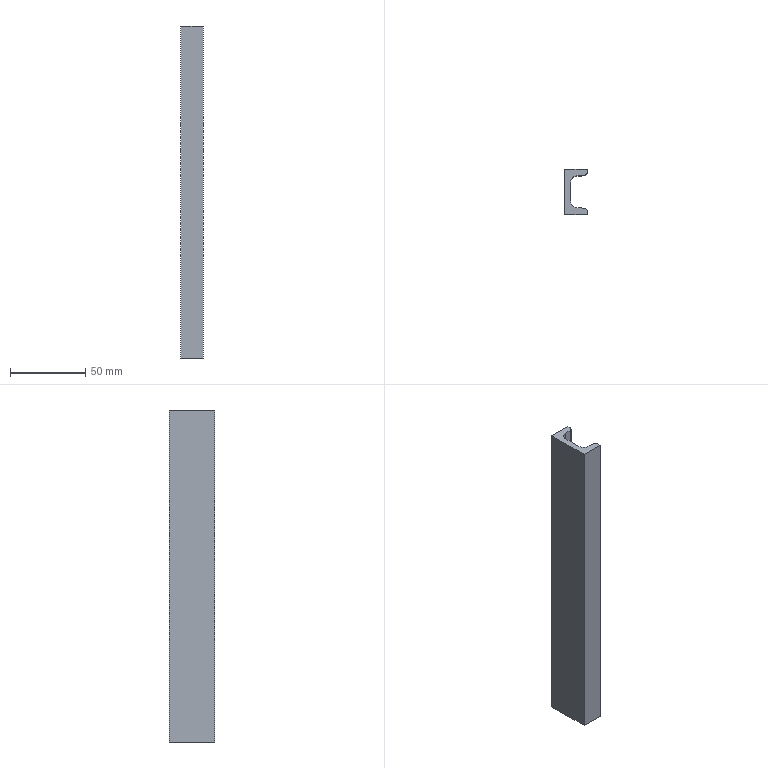Part | STEP file | DIN 1026-1 U 30x15 1785508252631 | 1 solid | 14 faces | box 15 x 30 x 220 mm | volume 48676 mm3 | plane 10 | cylinder 4 | commonest cylinder face diameters 4 x2 9 x2
STEP:
#1=CARTESIAN_POINT('',(4.,-6.066,220.));
#2=VERTEX_POINT('',#1);
#3=CARTESIAN_POINT('',(8.141,-10.551,220.));
#4=VERTEX_POINT('',#3);
#5=CARTESIAN_POINT('',(8.5,-6.066,220.));
#6=DIRECTION('',(0.,0.,1.));
#7=DIRECTION('',(-1.,0.,0.));
#8=AXIS2_PLACEMENT_3D('',#5,#6,#7);
#9=CIRCLE('',#8,4.5);
#10=EDGE_CURVE('',#2,#4,#9,.T.);
#11=ORIENTED_EDGE('',*,*,#10,.T.);
#12=CARTESIAN_POINT('',(8.141,-10.551,0.));
#13=VERTEX_POINT('',#12);
#14=CARTESIAN_POINT('',(8.141,-10.551,0.));
#15=DIRECTION('',(0.,0.,1.));
#16=VECTOR('',#15,10.);
#17=LINE('',#14,#16);
#18=EDGE_CURVE('',#13,#4,#17,.T.);
#19=ORIENTED_EDGE('',*,*,#18,.F.);
#20=CARTESIAN_POINT('',(4.,-6.066,0.));
#21=VERTEX_POINT('',#20);
#22=CARTESIAN_POINT('',(8.5,-6.066,0.));
#23=DIRECTION('',(0.,0.,1.));
#24=DIRECTION('',(-1.,0.,0.));
#25=AXIS2_PLACEMENT_3D('',#22,#23,#24);
#26=CIRCLE('',#25,4.5);
#27=EDGE_CURVE('',#21,#13,#26,.T.);
#28=ORIENTED_EDGE('',*,*,#27,.F.);
#29=CARTESIAN_POINT('',(4.,-6.066,0.));
#30=DIRECTION('',(0.,0.,1.));
#31=VECTOR('',#30,10.);
#32=LINE('',#29,#31);
#33=EDGE_CURVE('',#21,#2,#32,.T.);
#34=ORIENTED_EDGE('',*,*,#33,.T.);
#35=EDGE_LOOP('',(#11,#19,#28,#34));
#36=FACE_OUTER_BOUND('',#35,.T.);
#37=CARTESIAN_POINT('',(8.5,-6.066,0.));
#38=DIRECTION('',(0.,0.,1.));
#39=DIRECTION('',(-1.,0.,0.));
#40=AXIS2_PLACEMENT_3D('',#37,#38,#39);
#41=CYLINDRICAL_SURFACE('',#40,4.5);
#42=ADVANCED_FACE('',(#36),#41,.F.);
#43=CARTESIAN_POINT('',(13.159,-10.953,220.));
#44=VERTEX_POINT('',#43);
#45=CARTESIAN_POINT('',(7.403,-10.492,220.));
#46=DIRECTION('',(0.9968,-0.07975,0.));
#47=VECTOR('',#46,10.);
#48=LINE('',#45,#47);
#49=EDGE_CURVE('',#4,#44,#48,.T.);
#50=ORIENTED_EDGE('',*,*,#49,.T.);
#51=CARTESIAN_POINT('',(13.159,-10.953,0.));
#52=VERTEX_POINT('',#51);
#53=CARTESIAN_POINT('',(13.159,-10.953,0.));
#54=DIRECTION('',(0.,0.,1.));
#55=VECTOR('',#54,10.);
#56=LINE('',#53,#55);
#57=EDGE_CURVE('',#52,#44,#56,.T.);
#58=ORIENTED_EDGE('',*,*,#57,.F.);
#59=CARTESIAN_POINT('',(7.403,-10.492,0.));
#60=DIRECTION('',(0.9968,-0.07975,0.));
#61=VECTOR('',#60,10.);
#62=LINE('',#59,#61);
#63=EDGE_CURVE('',#13,#52,#62,.T.);
#64=ORIENTED_EDGE('',*,*,#63,.F.);
#65=ORIENTED_EDGE('',*,*,#18,.T.);
#66=EDGE_LOOP('',(#50,#58,#64,#65));
#67=FACE_OUTER_BOUND('',#66,.T.);
#68=CARTESIAN_POINT('',(8.141,-10.551,0.));
#69=DIRECTION('',(0.07975,0.9968,0.));
#70=DIRECTION('',(0.,0.,1.));
#71=AXIS2_PLACEMENT_3D('',#68,#69,#70);
#72=PLANE('',#71);
#73=ADVANCED_FACE('',(#67),#72,.T.);
#74=CARTESIAN_POINT('',(15.,-12.946,220.));
#75=VERTEX_POINT('',#74);
#76=CARTESIAN_POINT('',(13.,-12.946,220.));
#77=DIRECTION('',(0.,0.,-1.));
#78=DIRECTION('',(-1.,0.,0.));
#79=AXIS2_PLACEMENT_3D('',#76,#77,#78);
#80=CIRCLE('',#79,2.);
#81=EDGE_CURVE('',#44,#75,#80,.T.);
#82=ORIENTED_EDGE('',*,*,#81,.T.);
#83=CARTESIAN_POINT('',(15.,-12.946,0.));
#84=VERTEX_POINT('',#83);
#85=CARTESIAN_POINT('',(15.,-12.946,0.));
#86=DIRECTION('',(0.,0.,1.));
#87=VECTOR('',#86,10.);
#88=LINE('',#85,#87);
#89=EDGE_CURVE('',#84,#75,#88,.T.);
#90=ORIENTED_EDGE('',*,*,#89,.F.);
#91=CARTESIAN_POINT('',(13.,-12.946,0.));
#92=DIRECTION('',(0.,0.,-1.));
#93=DIRECTION('',(-1.,0.,0.));
#94=AXIS2_PLACEMENT_3D('',#91,#92,#93);
#95=CIRCLE('',#94,2.);
#96=EDGE_CURVE('',#52,#84,#95,.T.);
#97=ORIENTED_EDGE('',*,*,#96,.F.);
#98=ORIENTED_EDGE('',*,*,#57,.T.);
#99=EDGE_LOOP('',(#82,#90,#97,#98));
#100=FACE_OUTER_BOUND('',#99,.T.);
#101=CARTESIAN_POINT('',(13.,-12.946,0.));
#102=DIRECTION('',(0.,0.,1.));
#103=DIRECTION('',(-1.,0.,0.));
#104=AXIS2_PLACEMENT_3D('',#101,#102,#103);
#105=CYLINDRICAL_SURFACE('',#104,2.);
#106=ADVANCED_FACE('',(#100),#105,.T.);
#107=CARTESIAN_POINT('',(15.,-15.,220.));
#108=VERTEX_POINT('',#107);
#109=CARTESIAN_POINT('',(15.,-6.473,220.));
#110=DIRECTION('',(0.,-1.,0.));
#111=VECTOR('',#110,10.);
#112=LINE('',#109,#111);
#113=EDGE_CURVE('',#75,#108,#112,.T.);
#114=ORIENTED_EDGE('',*,*,#113,.T.);
#115=CARTESIAN_POINT('',(15.,-15.,0.));
#116=VERTEX_POINT('',#115);
#117=CARTESIAN_POINT('',(15.,-15.,0.));
#118=DIRECTION('',(0.,0.,1.));
#119=VECTOR('',#118,10.);
#120=LINE('',#117,#119);
#121=EDGE_CURVE('',#116,#108,#120,.T.);
#122=ORIENTED_EDGE('',*,*,#121,.F.);
#123=CARTESIAN_POINT('',(15.,-6.473,0.));
#124=DIRECTION('',(0.,-1.,0.));
#125=VECTOR('',#124,10.);
#126=LINE('',#123,#125);
#127=EDGE_CURVE('',#84,#116,#126,.T.);
#128=ORIENTED_EDGE('',*,*,#127,.F.);
#129=ORIENTED_EDGE('',*,*,#89,.T.);
#130=EDGE_LOOP('',(#114,#122,#128,#129));
#131=FACE_OUTER_BOUND('',#130,.T.);
#132=CARTESIAN_POINT('',(15.,-12.946,0.));
#133=DIRECTION('',(1.,0.,0.));
#134=DIRECTION('',(0.,0.,-1.));
#135=AXIS2_PLACEMENT_3D('',#132,#133,#134);
#136=PLANE('',#135);
#137=ADVANCED_FACE('',(#131),#136,.T.);
#138=CARTESIAN_POINT('',(0.,-15.,220.));
#139=VERTEX_POINT('',#138);
#140=CARTESIAN_POINT('',(11.25,-15.,220.));
#141=DIRECTION('',(-1.,0.,0.));
#142=VECTOR('',#141,10.);
#143=LINE('',#140,#142);
#144=EDGE_CURVE('',#108,#139,#143,.T.);
#145=ORIENTED_EDGE('',*,*,#144,.T.);
#146=CARTESIAN_POINT('',(0.,-15.,0.));
#147=VERTEX_POINT('',#146);
#148=CARTESIAN_POINT('',(0.,-15.,0.));
#149=DIRECTION('',(0.,0.,1.));
#150=VECTOR('',#149,10.);
#151=LINE('',#148,#150);
#152=EDGE_CURVE('',#147,#139,#151,.T.);
#153=ORIENTED_EDGE('',*,*,#152,.F.);
#154=CARTESIAN_POINT('',(11.25,-15.,0.));
#155=DIRECTION('',(-1.,0.,0.));
#156=VECTOR('',#155,10.);
#157=LINE('',#154,#156);
#158=EDGE_CURVE('',#116,#147,#157,.T.);
#159=ORIENTED_EDGE('',*,*,#158,.F.);
#160=ORIENTED_EDGE('',*,*,#121,.T.);
#161=EDGE_LOOP('',(#145,#153,#159,#160));
#162=FACE_OUTER_BOUND('',#161,.T.);
#163=CARTESIAN_POINT('',(15.,-15.,0.));
#164=DIRECTION('',(0.,-1.,0.));
#165=DIRECTION('',(0.,0.,-1.));
#166=AXIS2_PLACEMENT_3D('',#163,#164,#165);
#167=PLANE('',#166);
#168=ADVANCED_FACE('',(#162),#167,.T.);
#169=CARTESIAN_POINT('',(0.,15.,220.));
#170=VERTEX_POINT('',#169);
#171=CARTESIAN_POINT('',(0.,0.,220.));
#172=DIRECTION('',(0.,1.,0.));
#173=VECTOR('',#172,10.);
#174=LINE('',#171,#173);
#175=EDGE_CURVE('',#139,#170,#174,.T.);
#176=ORIENTED_EDGE('',*,*,#175,.T.);
#177=CARTESIAN_POINT('',(0.,15.,0.));
#178=VERTEX_POINT('',#177);
#179=CARTESIAN_POINT('',(0.,15.,0.));
#180=DIRECTION('',(0.,0.,1.));
#181=VECTOR('',#180,10.);
#182=LINE('',#179,#181);
#183=EDGE_CURVE('',#178,#170,#182,.T.);
#184=ORIENTED_EDGE('',*,*,#183,.F.);
#185=CARTESIAN_POINT('',(0.,0.,0.));
#186=DIRECTION('',(0.,1.,0.));
#187=VECTOR('',#186,10.);
#188=LINE('',#185,#187);
#189=EDGE_CURVE('',#147,#178,#188,.T.);
#190=ORIENTED_EDGE('',*,*,#189,.F.);
#191=ORIENTED_EDGE('',*,*,#152,.T.);
#192=EDGE_LOOP('',(#176,#184,#190,#191));
#193=FACE_OUTER_BOUND('',#192,.T.);
#194=CARTESIAN_POINT('',(0.,0.,0.));
#195=DIRECTION('',(-1.,0.,0.));
#196=DIRECTION('',(0.,0.,1.));
#197=AXIS2_PLACEMENT_3D('',#194,#195,#196);
#198=PLANE('',#197);
#199=ADVANCED_FACE('',(#193),#198,.T.);
#200=CARTESIAN_POINT('',(15.,15.,220.));
#201=VERTEX_POINT('',#200);
#202=CARTESIAN_POINT('',(3.75,15.,220.));
#203=DIRECTION('',(1.,0.,0.));
#204=VECTOR('',#203,10.);
#205=LINE('',#202,#204);
#206=EDGE_CURVE('',#170,#201,#205,.T.);
#207=ORIENTED_EDGE('',*,*,#206,.T.);
#208=CARTESIAN_POINT('',(15.,15.,0.));
#209=VERTEX_POINT('',#208);
#210=CARTESIAN_POINT('',(15.,15.,0.));
#211=DIRECTION('',(0.,0.,1.));
#212=VECTOR('',#211,10.);
#213=LINE('',#210,#212);
#214=EDGE_CURVE('',#209,#201,#213,.T.);
#215=ORIENTED_EDGE('',*,*,#214,.F.);
#216=CARTESIAN_POINT('',(3.75,15.,0.));
#217=DIRECTION('',(1.,0.,0.));
#218=VECTOR('',#217,10.);
#219=LINE('',#216,#218);
#220=EDGE_CURVE('',#178,#209,#219,.T.);
#221=ORIENTED_EDGE('',*,*,#220,.F.);
#222=ORIENTED_EDGE('',*,*,#183,.T.);
#223=EDGE_LOOP('',(#207,#215,#221,#222));
#224=FACE_OUTER_BOUND('',#223,.T.);
#225=CARTESIAN_POINT('',(0.,15.,0.));
#226=DIRECTION('',(0.,1.,0.));
#227=DIRECTION('',(0.,0.,1.));
#228=AXIS2_PLACEMENT_3D('',#225,#226,#227);
#229=PLANE('',#228);
#230=ADVANCED_FACE('',(#224),#229,.T.);
#231=CARTESIAN_POINT('',(15.,12.946,220.));
#232=VERTEX_POINT('',#231);
#233=CARTESIAN_POINT('',(15.,7.5,220.));
#234=DIRECTION('',(0.,-1.,0.));
#235=VECTOR('',#234,10.);
#236=LINE('',#233,#235);
#237=EDGE_CURVE('',#201,#232,#236,.T.);
#238=ORIENTED_EDGE('',*,*,#237,.T.);
#239=CARTESIAN_POINT('',(15.,12.946,0.));
#240=VERTEX_POINT('',#239);
#241=CARTESIAN_POINT('',(15.,12.946,0.));
#242=DIRECTION('',(0.,0.,1.));
#243=VECTOR('',#242,10.);
#244=LINE('',#241,#243);
#245=EDGE_CURVE('',#240,#232,#244,.T.);
#246=ORIENTED_EDGE('',*,*,#245,.F.);
#247=CARTESIAN_POINT('',(15.,7.5,0.));
#248=DIRECTION('',(0.,-1.,0.));
#249=VECTOR('',#248,10.);
#250=LINE('',#247,#249);
#251=EDGE_CURVE('',#209,#240,#250,.T.);
#252=ORIENTED_EDGE('',*,*,#251,.F.);
#253=ORIENTED_EDGE('',*,*,#214,.T.);
#254=EDGE_LOOP('',(#238,#246,#252,#253));
#255=FACE_OUTER_BOUND('',#254,.T.);
#256=CARTESIAN_POINT('',(15.,15.,0.));
#257=DIRECTION('',(1.,0.,0.));
#258=DIRECTION('',(0.,0.,-1.));
#259=AXIS2_PLACEMENT_3D('',#256,#257,#258);
#260=PLANE('',#259);
#261=ADVANCED_FACE('',(#255),#260,.T.);
#262=CARTESIAN_POINT('',(13.159,10.953,220.));
#263=VERTEX_POINT('',#262);
#264=CARTESIAN_POINT('',(13.,12.946,220.));
#265=DIRECTION('',(0.,0.,-1.));
#266=DIRECTION('',(-0.07975,0.9968,0.));
#267=AXIS2_PLACEMENT_3D('',#264,#265,#266);
#268=CIRCLE('',#267,2.);
#269=EDGE_CURVE('',#232,#263,#268,.T.);
#270=ORIENTED_EDGE('',*,*,#269,.T.);
#271=CARTESIAN_POINT('',(13.159,10.953,0.));
#272=VERTEX_POINT('',#271);
#273=CARTESIAN_POINT('',(13.159,10.953,0.));
#274=DIRECTION('',(0.,0.,1.));
#275=VECTOR('',#274,10.);
#276=LINE('',#273,#275);
#277=EDGE_CURVE('',#272,#263,#276,.T.);
#278=ORIENTED_EDGE('',*,*,#277,.F.);
#279=CARTESIAN_POINT('',(13.,12.946,0.));
#280=DIRECTION('',(0.,0.,-1.));
#281=DIRECTION('',(-0.07975,0.9968,0.));
#282=AXIS2_PLACEMENT_3D('',#279,#280,#281);
#283=CIRCLE('',#282,2.);
#284=EDGE_CURVE('',#240,#272,#283,.T.);
#285=ORIENTED_EDGE('',*,*,#284,.F.);
#286=ORIENTED_EDGE('',*,*,#245,.T.);
#287=EDGE_LOOP('',(#270,#278,#285,#286));
#288=FACE_OUTER_BOUND('',#287,.T.);
#289=CARTESIAN_POINT('',(13.,12.946,0.));
#290=DIRECTION('',(0.,0.,1.));
#291=DIRECTION('',(-0.07975,0.9968,0.));
#292=AXIS2_PLACEMENT_3D('',#289,#290,#291);
#293=CYLINDRICAL_SURFACE('',#292,2.);
#294=ADVANCED_FACE('',(#288),#293,.T.);
#295=CARTESIAN_POINT('',(8.141,10.551,220.));
#296=VERTEX_POINT('',#295);
#297=CARTESIAN_POINT('',(9.912,10.693,220.));
#298=DIRECTION('',(-0.9968,-0.07975,0.));
#299=VECTOR('',#298,10.);
#300=LINE('',#297,#299);
#301=EDGE_CURVE('',#263,#296,#300,.T.);
#302=ORIENTED_EDGE('',*,*,#301,.T.);
#303=CARTESIAN_POINT('',(8.141,10.551,0.));
#304=VERTEX_POINT('',#303);
#305=CARTESIAN_POINT('',(8.141,10.551,0.));
#306=DIRECTION('',(0.,0.,1.));
#307=VECTOR('',#306,10.);
#308=LINE('',#305,#307);
#309=EDGE_CURVE('',#304,#296,#308,.T.);
#310=ORIENTED_EDGE('',*,*,#309,.F.);
#311=CARTESIAN_POINT('',(9.912,10.693,0.));
#312=DIRECTION('',(-0.9968,-0.07975,0.));
#313=VECTOR('',#312,10.);
#314=LINE('',#311,#313);
#315=EDGE_CURVE('',#272,#304,#314,.T.);
#316=ORIENTED_EDGE('',*,*,#315,.F.);
#317=ORIENTED_EDGE('',*,*,#277,.T.);
#318=EDGE_LOOP('',(#302,#310,#316,#317));
#319=FACE_OUTER_BOUND('',#318,.T.);
#320=CARTESIAN_POINT('',(13.159,10.953,0.));
#321=DIRECTION('',(0.07975,-0.9968,0.));
#322=DIRECTION('',(0.,0.,-1.));
#323=AXIS2_PLACEMENT_3D('',#320,#321,#322);
#324=PLANE('',#323);
#325=ADVANCED_FACE('',(#319),#324,.T.);
#326=CARTESIAN_POINT('',(4.,6.066,220.));
#327=VERTEX_POINT('',#326);
#328=CARTESIAN_POINT('',(8.5,6.066,220.));
#329=DIRECTION('',(0.,0.,1.));
#330=DIRECTION('',(-0.07975,0.9968,0.));
#331=AXIS2_PLACEMENT_3D('',#328,#329,#330);
#332=CIRCLE('',#331,4.5);
#333=EDGE_CURVE('',#296,#327,#332,.T.);
#334=ORIENTED_EDGE('',*,*,#333,.T.);
#335=CARTESIAN_POINT('',(4.,6.066,0.));
#336=VERTEX_POINT('',#335);
#337=CARTESIAN_POINT('',(4.,6.066,0.));
#338=DIRECTION('',(0.,0.,1.));
#339=VECTOR('',#338,10.);
#340=LINE('',#337,#339);
#341=EDGE_CURVE('',#336,#327,#340,.T.);
#342=ORIENTED_EDGE('',*,*,#341,.F.);
#343=CARTESIAN_POINT('',(8.5,6.066,0.));
#344=DIRECTION('',(0.,0.,1.));
#345=DIRECTION('',(-0.07975,0.9968,0.));
#346=AXIS2_PLACEMENT_3D('',#343,#344,#345);
#347=CIRCLE('',#346,4.5);
#348=EDGE_CURVE('',#304,#336,#347,.T.);
#349=ORIENTED_EDGE('',*,*,#348,.F.);
#350=ORIENTED_EDGE('',*,*,#309,.T.);
#351=EDGE_LOOP('',(#334,#342,#349,#350));
#352=FACE_OUTER_BOUND('',#351,.T.);
#353=CARTESIAN_POINT('',(8.5,6.066,0.));
#354=DIRECTION('',(0.,0.,1.));
#355=DIRECTION('',(-0.07975,0.9968,0.));
#356=AXIS2_PLACEMENT_3D('',#353,#354,#355);
#357=CYLINDRICAL_SURFACE('',#356,4.5);
#358=ADVANCED_FACE('',(#352),#357,.F.);
#359=CARTESIAN_POINT('',(4.,0.,220.));
#360=DIRECTION('',(0.,-1.,0.));
#361=VECTOR('',#360,10.);
#362=LINE('',#359,#361);
#363=EDGE_CURVE('',#327,#2,#362,.T.);
#364=ORIENTED_EDGE('',*,*,#363,.T.);
#365=ORIENTED_EDGE('',*,*,#33,.F.);
#366=CARTESIAN_POINT('',(4.,0.,0.));
#367=DIRECTION('',(0.,-1.,0.));
#368=VECTOR('',#367,10.);
#369=LINE('',#366,#368);
#370=EDGE_CURVE('',#336,#21,#369,.T.);
#371=ORIENTED_EDGE('',*,*,#370,.F.);
#372=ORIENTED_EDGE('',*,*,#341,.T.);
#373=EDGE_LOOP('',(#364,#365,#371,#372));
#374=FACE_OUTER_BOUND('',#373,.T.);
#375=CARTESIAN_POINT('',(4.,0.,0.));
#376=DIRECTION('',(1.,0.,0.));
#377=DIRECTION('',(0.,0.,-1.));
#378=AXIS2_PLACEMENT_3D('',#375,#376,#377);
#379=PLANE('',#378);
#380=ADVANCED_FACE('',(#374),#379,.T.);
#381=ORIENTED_EDGE('',*,*,#220,.T.);
#382=ORIENTED_EDGE('',*,*,#251,.T.);
#383=ORIENTED_EDGE('',*,*,#284,.T.);
#384=ORIENTED_EDGE('',*,*,#315,.T.);
#385=ORIENTED_EDGE('',*,*,#348,.T.);
#386=ORIENTED_EDGE('',*,*,#370,.T.);
#387=ORIENTED_EDGE('',*,*,#27,.T.);
#388=ORIENTED_EDGE('',*,*,#63,.T.);
#389=ORIENTED_EDGE('',*,*,#96,.T.);
#390=ORIENTED_EDGE('',*,*,#127,.T.);
#391=ORIENTED_EDGE('',*,*,#158,.T.);
#392=ORIENTED_EDGE('',*,*,#189,.T.);
#393=EDGE_LOOP('',(#381,#382,#383,#384,#385,#386,#387,#388,#389,#390,#391,#392));
#394=FACE_OUTER_BOUND('',#393,.T.);
#395=CARTESIAN_POINT('',(7.5,0.,0.));
#396=DIRECTION('',(0.,0.,1.));
#397=DIRECTION('',(1.,0.,0.));
#398=AXIS2_PLACEMENT_3D('',#395,#396,#397);
#399=PLANE('',#398);
#400=ADVANCED_FACE('',(#394),#399,.F.);
#401=ORIENTED_EDGE('',*,*,#206,.F.);
#402=ORIENTED_EDGE('',*,*,#175,.F.);
#403=ORIENTED_EDGE('',*,*,#144,.F.);
#404=ORIENTED_EDGE('',*,*,#113,.F.);
#405=ORIENTED_EDGE('',*,*,#81,.F.);
#406=ORIENTED_EDGE('',*,*,#49,.F.);
#407=ORIENTED_EDGE('',*,*,#10,.F.);
#408=ORIENTED_EDGE('',*,*,#363,.F.);
#409=ORIENTED_EDGE('',*,*,#333,.F.);
#410=ORIENTED_EDGE('',*,*,#301,.F.);
#411=ORIENTED_EDGE('',*,*,#269,.F.);
#412=ORIENTED_EDGE('',*,*,#237,.F.);
#413=EDGE_LOOP('',(#401,#402,#403,#404,#405,#406,#407,#408,#409,#410,#411,#412));
#414=FACE_OUTER_BOUND('',#413,.T.);
#415=CARTESIAN_POINT('',(7.5,0.,220.));
#416=DIRECTION('',(0.,0.,1.));
#417=DIRECTION('',(1.,0.,0.));
#418=AXIS2_PLACEMENT_3D('',#415,#416,#417);
#419=PLANE('',#418);
#420=ADVANCED_FACE('',(#414),#419,.T.);
#421=CLOSED_SHELL('',(#42,#73,#106,#137,#168,#199,#230,#261,#294,#325,#358,#380,#400,#420));
#422=MANIFOLD_SOLID_BREP('',#421);
#423=(LENGTH_UNIT()NAMED_UNIT(*)SI_UNIT(.MILLI.,.METRE.));
#424=UNCERTAINTY_MEASURE_WITH_UNIT(LENGTH_MEASURE(0.01),#423,'','');
#425=(NAMED_UNIT(*)PLANE_ANGLE_UNIT()SI_UNIT($,.RADIAN.));
#426=(NAMED_UNIT(*)SI_UNIT($,.STERADIAN.)SOLID_ANGLE_UNIT());
#427=(GEOMETRIC_REPRESENTATION_CONTEXT(3)GLOBAL_UNCERTAINTY_ASSIGNED_CONTEXT((#424))GLOBAL_UNIT_ASSIGNED_CONTEXT((#423,#425,#426))REPRESENTATION_CONTEXT('',''));
#428=ADVANCED_BREP_SHAPE_REPRESENTATION('',(#422),#427);